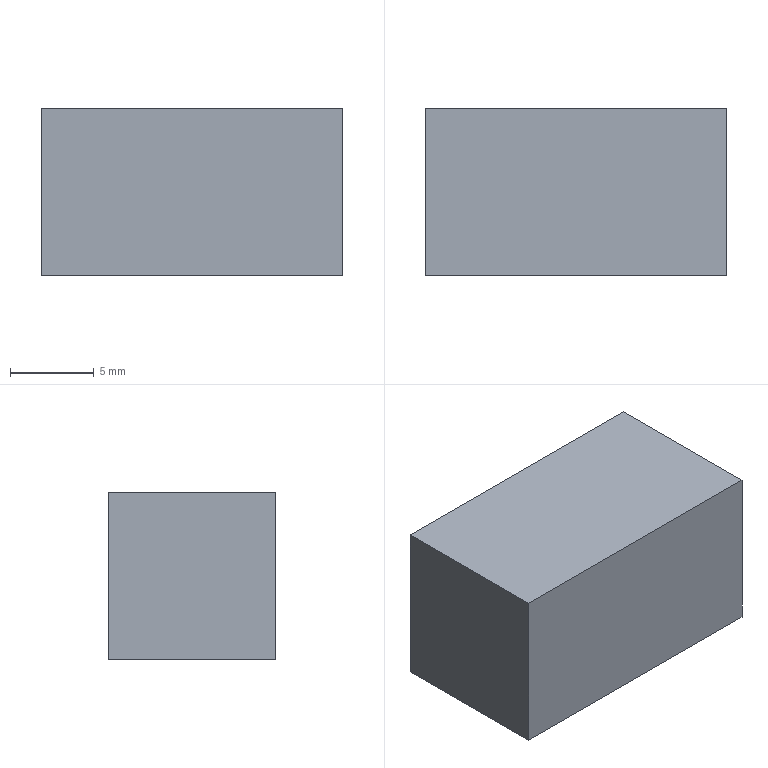Part | SolidWorks | features Extrusion 1 | 1 solid | 6 faces | box 18 x 10 x 10 mm | volume 1800 mm3 | plane 6
STEP:
#1=CARTESIAN_POINT('',(-9.,5.,5.));
#2=VERTEX_POINT('',#1);
#3=CARTESIAN_POINT('',(-9.,-5.,5.));
#4=VERTEX_POINT('',#3);
#5=CARTESIAN_POINT('',(-9.,5.,5.));
#6=DIRECTION('',(0.,-1.,0.));
#7=VECTOR('',#6,1000.);
#8=LINE('',#5,#7);
#9=EDGE_CURVE('',#2,#4,#8,.T.);
#10=ORIENTED_EDGE('',*,*,#9,.F.);
#11=CARTESIAN_POINT('',(-9.,5.,-5.));
#12=VERTEX_POINT('',#11);
#13=CARTESIAN_POINT('',(-9.,5.,-5.));
#14=DIRECTION('',(0.,0.,1.));
#15=VECTOR('',#14,1000.);
#16=LINE('',#13,#15);
#17=EDGE_CURVE('',#12,#2,#16,.T.);
#18=ORIENTED_EDGE('',*,*,#17,.F.);
#19=CARTESIAN_POINT('',(-9.,-5.,-5.));
#20=VERTEX_POINT('',#19);
#21=CARTESIAN_POINT('',(-9.,5.,-5.));
#22=DIRECTION('',(0.,-1.,0.));
#23=VECTOR('',#22,1000.);
#24=LINE('',#21,#23);
#25=EDGE_CURVE('',#12,#20,#24,.T.);
#26=ORIENTED_EDGE('',*,*,#25,.T.);
#27=CARTESIAN_POINT('',(-9.,-5.,-5.));
#28=DIRECTION('',(0.,0.,1.));
#29=VECTOR('',#28,1000.);
#30=LINE('',#27,#29);
#31=EDGE_CURVE('',#20,#4,#30,.T.);
#32=ORIENTED_EDGE('',*,*,#31,.T.);
#33=EDGE_LOOP('',(#10,#18,#26,#32));
#34=FACE_OUTER_BOUND('',#33,.T.);
#35=CARTESIAN_POINT('',(-9.,5.,-5.));
#36=DIRECTION('',(-1.,0.,0.));
#37=DIRECTION('',(0.,0.,1.));
#38=AXIS2_PLACEMENT_3D('',#35,#36,#37);
#39=PLANE('',#38);
#40=ADVANCED_FACE('',(#34),#39,.T.);
#41=CARTESIAN_POINT('',(9.,5.,5.));
#42=VERTEX_POINT('',#41);
#43=CARTESIAN_POINT('',(9.,5.,5.));
#44=DIRECTION('',(-1.,0.,0.));
#45=VECTOR('',#44,1000.);
#46=LINE('',#43,#45);
#47=EDGE_CURVE('',#42,#2,#46,.T.);
#48=ORIENTED_EDGE('',*,*,#47,.F.);
#49=CARTESIAN_POINT('',(9.,5.,-5.));
#50=VERTEX_POINT('',#49);
#51=CARTESIAN_POINT('',(9.,5.,-5.));
#52=DIRECTION('',(0.,0.,1.));
#53=VECTOR('',#52,1000.);
#54=LINE('',#51,#53);
#55=EDGE_CURVE('',#50,#42,#54,.T.);
#56=ORIENTED_EDGE('',*,*,#55,.F.);
#57=CARTESIAN_POINT('',(9.,5.,-5.));
#58=DIRECTION('',(-1.,0.,0.));
#59=VECTOR('',#58,1000.);
#60=LINE('',#57,#59);
#61=EDGE_CURVE('',#50,#12,#60,.T.);
#62=ORIENTED_EDGE('',*,*,#61,.T.);
#63=ORIENTED_EDGE('',*,*,#17,.T.);
#64=EDGE_LOOP('',(#48,#56,#62,#63));
#65=FACE_OUTER_BOUND('',#64,.T.);
#66=CARTESIAN_POINT('',(9.,5.,-5.));
#67=DIRECTION('',(0.,1.,0.));
#68=DIRECTION('',(0.,0.,1.));
#69=AXIS2_PLACEMENT_3D('',#66,#67,#68);
#70=PLANE('',#69);
#71=ADVANCED_FACE('',(#65),#70,.T.);
#72=CARTESIAN_POINT('',(9.,-5.,5.));
#73=VERTEX_POINT('',#72);
#74=CARTESIAN_POINT('',(9.,-5.,5.));
#75=DIRECTION('',(0.,1.,0.));
#76=VECTOR('',#75,1000.);
#77=LINE('',#74,#76);
#78=EDGE_CURVE('',#73,#42,#77,.T.);
#79=ORIENTED_EDGE('',*,*,#78,.F.);
#80=CARTESIAN_POINT('',(9.,-5.,-5.));
#81=VERTEX_POINT('',#80);
#82=CARTESIAN_POINT('',(9.,-5.,-5.));
#83=DIRECTION('',(0.,0.,1.));
#84=VECTOR('',#83,1000.);
#85=LINE('',#82,#84);
#86=EDGE_CURVE('',#81,#73,#85,.T.);
#87=ORIENTED_EDGE('',*,*,#86,.F.);
#88=CARTESIAN_POINT('',(9.,-5.,-5.));
#89=DIRECTION('',(0.,1.,0.));
#90=VECTOR('',#89,1000.);
#91=LINE('',#88,#90);
#92=EDGE_CURVE('',#81,#50,#91,.T.);
#93=ORIENTED_EDGE('',*,*,#92,.T.);
#94=ORIENTED_EDGE('',*,*,#55,.T.);
#95=EDGE_LOOP('',(#79,#87,#93,#94));
#96=FACE_OUTER_BOUND('',#95,.T.);
#97=CARTESIAN_POINT('',(9.,-5.,-5.));
#98=DIRECTION('',(1.,0.,0.));
#99=DIRECTION('',(0.,0.,-1.));
#100=AXIS2_PLACEMENT_3D('',#97,#98,#99);
#101=PLANE('',#100);
#102=ADVANCED_FACE('',(#96),#101,.T.);
#103=CARTESIAN_POINT('',(-9.,-5.,5.));
#104=DIRECTION('',(1.,0.,0.));
#105=VECTOR('',#104,1000.);
#106=LINE('',#103,#105);
#107=EDGE_CURVE('',#4,#73,#106,.T.);
#108=ORIENTED_EDGE('',*,*,#107,.F.);
#109=ORIENTED_EDGE('',*,*,#31,.F.);
#110=CARTESIAN_POINT('',(-9.,-5.,-5.));
#111=DIRECTION('',(1.,0.,0.));
#112=VECTOR('',#111,1000.);
#113=LINE('',#110,#112);
#114=EDGE_CURVE('',#20,#81,#113,.T.);
#115=ORIENTED_EDGE('',*,*,#114,.T.);
#116=ORIENTED_EDGE('',*,*,#86,.T.);
#117=EDGE_LOOP('',(#108,#109,#115,#116));
#118=FACE_OUTER_BOUND('',#117,.T.);
#119=CARTESIAN_POINT('',(-9.,-5.,-5.));
#120=DIRECTION('',(0.,-1.,0.));
#121=DIRECTION('',(0.,0.,-1.));
#122=AXIS2_PLACEMENT_3D('',#119,#120,#121);
#123=PLANE('',#122);
#124=ADVANCED_FACE('',(#118),#123,.T.);
#125=ORIENTED_EDGE('',*,*,#25,.F.);
#126=ORIENTED_EDGE('',*,*,#61,.F.);
#127=ORIENTED_EDGE('',*,*,#92,.F.);
#128=ORIENTED_EDGE('',*,*,#114,.F.);
#129=EDGE_LOOP('',(#125,#126,#127,#128));
#130=FACE_OUTER_BOUND('',#129,.T.);
#131=CARTESIAN_POINT('',(0.,0.,-5.));
#132=DIRECTION('',(0.,0.,1.));
#133=DIRECTION('',(1.,0.,0.));
#134=AXIS2_PLACEMENT_3D('',#131,#132,#133);
#135=PLANE('',#134);
#136=ADVANCED_FACE('',(#130),#135,.F.);
#137=ORIENTED_EDGE('',*,*,#9,.T.);
#138=ORIENTED_EDGE('',*,*,#107,.T.);
#139=ORIENTED_EDGE('',*,*,#78,.T.);
#140=ORIENTED_EDGE('',*,*,#47,.T.);
#141=EDGE_LOOP('',(#137,#138,#139,#140));
#142=FACE_OUTER_BOUND('',#141,.T.);
#143=CARTESIAN_POINT('',(0.,0.,5.));
#144=DIRECTION('',(0.,0.,1.));
#145=DIRECTION('',(1.,0.,0.));
#146=AXIS2_PLACEMENT_3D('',#143,#144,#145);
#147=PLANE('',#146);
#148=ADVANCED_FACE('',(#142),#147,.T.);
#149=CLOSED_SHELL('',(#40,#71,#102,#124,#136,#148));
#150=MANIFOLD_SOLID_BREP('',#149);
#151=CARTESIAN_POINT('',(0.,0.,0.));
#152=DIRECTION('',(0.,0.,1.));
#153=DIRECTION('',(1.,0.,0.));
#154=AXIS2_PLACEMENT_3D('',#151,#152,#153);
#155=(LENGTH_UNIT()NAMED_UNIT(*)SI_UNIT(.MILLI.,.METRE.));
#156=UNCERTAINTY_MEASURE_WITH_UNIT(LENGTH_MEASURE(0.00001),#155,'','');
#157=(NAMED_UNIT(*)PLANE_ANGLE_UNIT()SI_UNIT($,.RADIAN.));
#158=(NAMED_UNIT(*)SI_UNIT($,.STERADIAN.)SOLID_ANGLE_UNIT());
#159=(GEOMETRIC_REPRESENTATION_CONTEXT(3)GLOBAL_UNCERTAINTY_ASSIGNED_CONTEXT((#156))GLOBAL_UNIT_ASSIGNED_CONTEXT((#155,#157,#158))REPRESENTATION_CONTEXT('',''));
#160=ADVANCED_BREP_SHAPE_REPRESENTATION('',(#150,#154),#159);